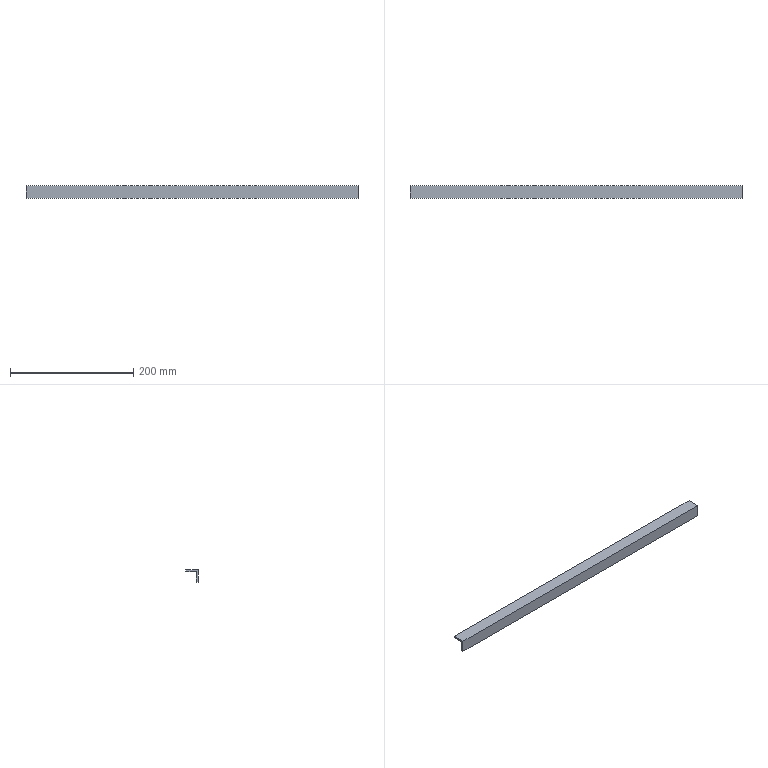Part | NX | 1 solid | 8 faces | box 538 x 20 x 20 mm | volume 59718 mm3 | plane 8
STEP:
#1=CARTESIAN_POINT('',(0.,0.,0.));
#2=VERTEX_POINT('',#1);
#3=CARTESIAN_POINT('',(0.,0.,-20.));
#4=VERTEX_POINT('',#3);
#5=CARTESIAN_POINT('',(0.,0.,0.));
#6=DIRECTION('',(0.,0.,-1.));
#7=VECTOR('',#6,1.);
#8=LINE('',#5,#7);
#9=EDGE_CURVE('',#2,#4,#8,.T.);
#10=ORIENTED_EDGE('',*,*,#9,.T.);
#11=CARTESIAN_POINT('',(538.,0.,-20.));
#12=VERTEX_POINT('',#11);
#13=CARTESIAN_POINT('',(538.,0.,-20.));
#14=DIRECTION('',(-1.,0.,0.));
#15=VECTOR('',#14,1.);
#16=LINE('',#13,#15);
#17=EDGE_CURVE('',#12,#4,#16,.T.);
#18=ORIENTED_EDGE('',*,*,#17,.F.);
#19=CARTESIAN_POINT('',(538.,0.,0.));
#20=VERTEX_POINT('',#19);
#21=CARTESIAN_POINT('',(538.,0.,0.));
#22=DIRECTION('',(0.,0.,-1.));
#23=VECTOR('',#22,1.);
#24=LINE('',#21,#23);
#25=EDGE_CURVE('',#20,#12,#24,.T.);
#26=ORIENTED_EDGE('',*,*,#25,.F.);
#27=CARTESIAN_POINT('',(538.,0.,0.));
#28=DIRECTION('',(-1.,0.,0.));
#29=VECTOR('',#28,1.);
#30=LINE('',#27,#29);
#31=EDGE_CURVE('',#20,#2,#30,.T.);
#32=ORIENTED_EDGE('',*,*,#31,.T.);
#33=EDGE_LOOP('',(#10,#18,#26,#32));
#34=FACE_OUTER_BOUND('',#33,.T.);
#35=CARTESIAN_POINT('',(538.,0.,0.));
#36=DIRECTION('',(0.,1.,0.));
#37=DIRECTION('',(0.,0.,1.));
#38=AXIS2_PLACEMENT_3D('',#35,#36,#37);
#39=PLANE('',#38);
#40=ADVANCED_FACE('',(#34),#39,.F.);
#41=CARTESIAN_POINT('',(0.,3.,-20.));
#42=VERTEX_POINT('',#41);
#43=CARTESIAN_POINT('',(0.,3.,-20.));
#44=DIRECTION('',(0.,1.,0.));
#45=VECTOR('',#44,1.);
#46=LINE('',#43,#45);
#47=EDGE_CURVE('',#4,#42,#46,.T.);
#48=ORIENTED_EDGE('',*,*,#47,.T.);
#49=CARTESIAN_POINT('',(538.,3.,-20.));
#50=VERTEX_POINT('',#49);
#51=CARTESIAN_POINT('',(538.,3.,-20.));
#52=DIRECTION('',(-1.,0.,0.));
#53=VECTOR('',#52,1.);
#54=LINE('',#51,#53);
#55=EDGE_CURVE('',#50,#42,#54,.T.);
#56=ORIENTED_EDGE('',*,*,#55,.F.);
#57=CARTESIAN_POINT('',(538.,3.,-20.));
#58=DIRECTION('',(0.,1.,0.));
#59=VECTOR('',#58,1.);
#60=LINE('',#57,#59);
#61=EDGE_CURVE('',#12,#50,#60,.T.);
#62=ORIENTED_EDGE('',*,*,#61,.F.);
#63=ORIENTED_EDGE('',*,*,#17,.T.);
#64=EDGE_LOOP('',(#48,#56,#62,#63));
#65=FACE_OUTER_BOUND('',#64,.T.);
#66=CARTESIAN_POINT('',(538.,3.,-20.));
#67=DIRECTION('',(0.,0.,1.));
#68=DIRECTION('',(1.,0.,0.));
#69=AXIS2_PLACEMENT_3D('',#66,#67,#68);
#70=PLANE('',#69);
#71=ADVANCED_FACE('',(#65),#70,.F.);
#72=CARTESIAN_POINT('',(0.,3.,-3.));
#73=VERTEX_POINT('',#72);
#74=CARTESIAN_POINT('',(0.,3.,-3.));
#75=DIRECTION('',(0.,0.,1.));
#76=VECTOR('',#75,1.);
#77=LINE('',#74,#76);
#78=EDGE_CURVE('',#42,#73,#77,.T.);
#79=ORIENTED_EDGE('',*,*,#78,.T.);
#80=CARTESIAN_POINT('',(538.,3.,-3.));
#81=VERTEX_POINT('',#80);
#82=CARTESIAN_POINT('',(538.,3.,-3.));
#83=DIRECTION('',(-1.,0.,0.));
#84=VECTOR('',#83,1.);
#85=LINE('',#82,#84);
#86=EDGE_CURVE('',#81,#73,#85,.T.);
#87=ORIENTED_EDGE('',*,*,#86,.F.);
#88=CARTESIAN_POINT('',(538.,3.,-3.));
#89=DIRECTION('',(0.,0.,1.));
#90=VECTOR('',#89,1.);
#91=LINE('',#88,#90);
#92=EDGE_CURVE('',#50,#81,#91,.T.);
#93=ORIENTED_EDGE('',*,*,#92,.F.);
#94=ORIENTED_EDGE('',*,*,#55,.T.);
#95=EDGE_LOOP('',(#79,#87,#93,#94));
#96=FACE_OUTER_BOUND('',#95,.T.);
#97=CARTESIAN_POINT('',(538.,3.,-3.));
#98=DIRECTION('',(0.,-1.,0.));
#99=DIRECTION('',(0.,0.,-1.));
#100=AXIS2_PLACEMENT_3D('',#97,#98,#99);
#101=PLANE('',#100);
#102=ADVANCED_FACE('',(#96),#101,.F.);
#103=CARTESIAN_POINT('',(0.,20.,-3.));
#104=VERTEX_POINT('',#103);
#105=CARTESIAN_POINT('',(0.,3.,-3.));
#106=DIRECTION('',(0.,1.,0.));
#107=VECTOR('',#106,1.);
#108=LINE('',#105,#107);
#109=EDGE_CURVE('',#73,#104,#108,.T.);
#110=ORIENTED_EDGE('',*,*,#109,.T.);
#111=CARTESIAN_POINT('',(538.,20.,-3.));
#112=VERTEX_POINT('',#111);
#113=CARTESIAN_POINT('',(538.,20.,-3.));
#114=DIRECTION('',(-1.,0.,0.));
#115=VECTOR('',#114,1.);
#116=LINE('',#113,#115);
#117=EDGE_CURVE('',#112,#104,#116,.T.);
#118=ORIENTED_EDGE('',*,*,#117,.F.);
#119=CARTESIAN_POINT('',(538.,3.,-3.));
#120=DIRECTION('',(0.,1.,0.));
#121=VECTOR('',#120,1.);
#122=LINE('',#119,#121);
#123=EDGE_CURVE('',#81,#112,#122,.T.);
#124=ORIENTED_EDGE('',*,*,#123,.F.);
#125=ORIENTED_EDGE('',*,*,#86,.T.);
#126=EDGE_LOOP('',(#110,#118,#124,#125));
#127=FACE_OUTER_BOUND('',#126,.T.);
#128=CARTESIAN_POINT('',(538.,3.,-3.));
#129=DIRECTION('',(0.,0.,1.));
#130=DIRECTION('',(1.,0.,0.));
#131=AXIS2_PLACEMENT_3D('',#128,#129,#130);
#132=PLANE('',#131);
#133=ADVANCED_FACE('',(#127),#132,.F.);
#134=CARTESIAN_POINT('',(0.,20.,0.));
#135=VERTEX_POINT('',#134);
#136=CARTESIAN_POINT('',(0.,20.,-3.));
#137=DIRECTION('',(0.,0.,1.));
#138=VECTOR('',#137,1.);
#139=LINE('',#136,#138);
#140=EDGE_CURVE('',#104,#135,#139,.T.);
#141=ORIENTED_EDGE('',*,*,#140,.T.);
#142=CARTESIAN_POINT('',(538.,20.,0.));
#143=VERTEX_POINT('',#142);
#144=CARTESIAN_POINT('',(538.,20.,0.));
#145=DIRECTION('',(-1.,0.,0.));
#146=VECTOR('',#145,1.);
#147=LINE('',#144,#146);
#148=EDGE_CURVE('',#143,#135,#147,.T.);
#149=ORIENTED_EDGE('',*,*,#148,.F.);
#150=CARTESIAN_POINT('',(538.,20.,-3.));
#151=DIRECTION('',(0.,0.,1.));
#152=VECTOR('',#151,1.);
#153=LINE('',#150,#152);
#154=EDGE_CURVE('',#112,#143,#153,.T.);
#155=ORIENTED_EDGE('',*,*,#154,.F.);
#156=ORIENTED_EDGE('',*,*,#117,.T.);
#157=EDGE_LOOP('',(#141,#149,#155,#156));
#158=FACE_OUTER_BOUND('',#157,.T.);
#159=CARTESIAN_POINT('',(538.,20.,-3.));
#160=DIRECTION('',(0.,-1.,0.));
#161=DIRECTION('',(0.,0.,-1.));
#162=AXIS2_PLACEMENT_3D('',#159,#160,#161);
#163=PLANE('',#162);
#164=ADVANCED_FACE('',(#158),#163,.F.);
#165=CARTESIAN_POINT('',(0.,0.,0.));
#166=DIRECTION('',(0.,-1.,0.));
#167=VECTOR('',#166,1.);
#168=LINE('',#165,#167);
#169=EDGE_CURVE('',#135,#2,#168,.T.);
#170=ORIENTED_EDGE('',*,*,#169,.T.);
#171=ORIENTED_EDGE('',*,*,#31,.F.);
#172=CARTESIAN_POINT('',(538.,0.,0.));
#173=DIRECTION('',(0.,-1.,0.));
#174=VECTOR('',#173,1.);
#175=LINE('',#172,#174);
#176=EDGE_CURVE('',#143,#20,#175,.T.);
#177=ORIENTED_EDGE('',*,*,#176,.F.);
#178=ORIENTED_EDGE('',*,*,#148,.T.);
#179=EDGE_LOOP('',(#170,#171,#177,#178));
#180=FACE_OUTER_BOUND('',#179,.T.);
#181=CARTESIAN_POINT('',(538.,0.,0.));
#182=DIRECTION('',(0.,0.,-1.));
#183=DIRECTION('',(-1.,0.,0.));
#184=AXIS2_PLACEMENT_3D('',#181,#182,#183);
#185=PLANE('',#184);
#186=ADVANCED_FACE('',(#180),#185,.F.);
#187=ORIENTED_EDGE('',*,*,#25,.T.);
#188=ORIENTED_EDGE('',*,*,#61,.T.);
#189=ORIENTED_EDGE('',*,*,#92,.T.);
#190=ORIENTED_EDGE('',*,*,#123,.T.);
#191=ORIENTED_EDGE('',*,*,#154,.T.);
#192=ORIENTED_EDGE('',*,*,#176,.T.);
#193=EDGE_LOOP('',(#187,#188,#189,#190,#191,#192));
#194=FACE_OUTER_BOUND('',#193,.T.);
#195=CARTESIAN_POINT('',(538.,0.,-20.));
#196=DIRECTION('',(-1.,0.,0.));
#197=DIRECTION('',(0.,0.,1.));
#198=AXIS2_PLACEMENT_3D('',#195,#196,#197);
#199=PLANE('',#198);
#200=ADVANCED_FACE('',(#194),#199,.F.);
#201=ORIENTED_EDGE('',*,*,#9,.F.);
#202=ORIENTED_EDGE('',*,*,#169,.F.);
#203=ORIENTED_EDGE('',*,*,#140,.F.);
#204=ORIENTED_EDGE('',*,*,#109,.F.);
#205=ORIENTED_EDGE('',*,*,#78,.F.);
#206=ORIENTED_EDGE('',*,*,#47,.F.);
#207=EDGE_LOOP('',(#201,#202,#203,#204,#205,#206));
#208=FACE_OUTER_BOUND('',#207,.T.);
#209=CARTESIAN_POINT('',(0.,0.,-20.));
#210=DIRECTION('',(-1.,0.,0.));
#211=DIRECTION('',(0.,0.,1.));
#212=AXIS2_PLACEMENT_3D('',#209,#210,#211);
#213=PLANE('',#212);
#214=ADVANCED_FACE('',(#208),#213,.T.);
#215=CLOSED_SHELL('',(#40,#71,#102,#133,#164,#186,#200,#214));
#216=MANIFOLD_SOLID_BREP('',#215);
#217=(LENGTH_UNIT()NAMED_UNIT(*)SI_UNIT(.MILLI.,.METRE.));
#218=UNCERTAINTY_MEASURE_WITH_UNIT(LENGTH_MEASURE(0.00002),#217,'','');
#219=(NAMED_UNIT(*)PLANE_ANGLE_UNIT()SI_UNIT($,.RADIAN.));
#220=PLANE_ANGLE_MEASURE_WITH_UNIT(PLANE_ANGLE_MEASURE(0.01745),#219);
#221=DIMENSIONAL_EXPONENTS(0.,0.,0.,0.,0.,0.,0.);
#222=(CONVERSION_BASED_UNIT('DEGREE',#220)NAMED_UNIT(#221)PLANE_ANGLE_UNIT());
#223=(NAMED_UNIT(*)SI_UNIT($,.STERADIAN.)SOLID_ANGLE_UNIT());
#224=(GEOMETRIC_REPRESENTATION_CONTEXT(3)GLOBAL_UNCERTAINTY_ASSIGNED_CONTEXT((#218))GLOBAL_UNIT_ASSIGNED_CONTEXT((#217,#222,#223))REPRESENTATION_CONTEXT('',''));
#225=ADVANCED_BREP_SHAPE_REPRESENTATION('',(#216),#224);